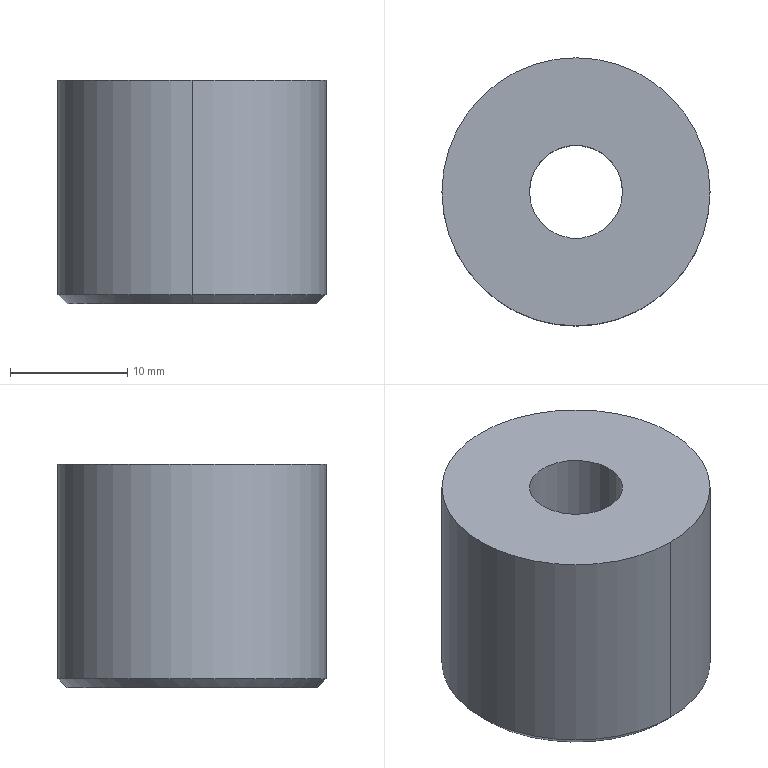Part | NX | features BREP 1 | 1 solid | 8 faces | box 22.86 x 22.86 x 19.05 mm | volume 6856 mm3 | cylinder 4 | plane 2 | cone 2 | commonest cylinder face diameters 7.938 x2 22.86 x2
STEP:
#1=CARTESIAN_POINT('',(0.,11.43,0.));
#2=VERTEX_POINT('',#1);
#3=CARTESIAN_POINT('',(0.,-11.43,0.));
#4=VERTEX_POINT('',#3);
#5=CARTESIAN_POINT('',(0.,0.,0.));
#6=DIRECTION('',(0.,0.,-1.));
#7=DIRECTION('',(0.,1.,0.));
#8=AXIS2_PLACEMENT_3D('',#5,#6,#7);
#9=CIRCLE('',#8,11.43);
#10=EDGE_CURVE('',#2,#4,#9,.T.);
#11=ORIENTED_EDGE('',*,*,#10,.F.);
#12=CARTESIAN_POINT('',(0.,0.,0.));
#13=DIRECTION('',(0.,0.,-1.));
#14=DIRECTION('',(0.,-1.,0.));
#15=AXIS2_PLACEMENT_3D('',#12,#13,#14);
#16=CIRCLE('',#15,11.43);
#17=EDGE_CURVE('',#4,#2,#16,.T.);
#18=ORIENTED_EDGE('',*,*,#17,.F.);
#19=EDGE_LOOP('',(#11,#18));
#20=FACE_BOUND('',#19,.T.);
#21=CARTESIAN_POINT('',(3.969,0.,0.));
#22=VERTEX_POINT('',#21);
#23=CARTESIAN_POINT('',(-3.969,0.,0.));
#24=VERTEX_POINT('',#23);
#25=CARTESIAN_POINT('',(0.,0.,0.));
#26=DIRECTION('',(0.,0.,-1.));
#27=DIRECTION('',(1.,0.,0.));
#28=AXIS2_PLACEMENT_3D('',#25,#26,#27);
#29=CIRCLE('',#28,3.969);
#30=EDGE_CURVE('',#22,#24,#29,.T.);
#31=ORIENTED_EDGE('',*,*,#30,.T.);
#32=CARTESIAN_POINT('',(0.,0.,0.));
#33=DIRECTION('',(0.,0.,-1.));
#34=DIRECTION('',(-1.,0.,0.));
#35=AXIS2_PLACEMENT_3D('',#32,#33,#34);
#36=CIRCLE('',#35,3.969);
#37=EDGE_CURVE('',#24,#22,#36,.T.);
#38=ORIENTED_EDGE('',*,*,#37,.T.);
#39=EDGE_LOOP('',(#31,#38));
#40=FACE_BOUND('',#39,.T.);
#41=CARTESIAN_POINT('',(0.,0.,0.));
#42=DIRECTION('',(0.,0.,-1.));
#43=DIRECTION('',(0.,-1.,0.));
#44=AXIS2_PLACEMENT_3D('',#41,#42,#43);
#45=PLANE('',#44);
#46=ADVANCED_FACE('',(#20,#40),#45,.F.);
#47=CARTESIAN_POINT('',(0.,11.43,-18.288));
#48=VERTEX_POINT('',#47);
#49=CARTESIAN_POINT('',(0.,11.43,0.));
#50=DIRECTION('',(0.,0.,-1.));
#51=VECTOR('',#50,1000.);
#52=LINE('',#49,#51);
#53=EDGE_CURVE('',#48,#2,#52,.F.);
#54=ORIENTED_EDGE('',*,*,#53,.F.);
#55=CARTESIAN_POINT('',(0.,-11.43,-18.288));
#56=VERTEX_POINT('',#55);
#57=CARTESIAN_POINT('',(0.,0.,-18.288));
#58=DIRECTION('',(0.,0.,-1.));
#59=DIRECTION('',(0.,-1.,0.));
#60=AXIS2_PLACEMENT_3D('',#57,#58,#59);
#61=CIRCLE('',#60,11.43);
#62=EDGE_CURVE('',#56,#48,#61,.T.);
#63=ORIENTED_EDGE('',*,*,#62,.F.);
#64=CARTESIAN_POINT('',(0.,-11.43,0.));
#65=DIRECTION('',(0.,0.,-1.));
#66=VECTOR('',#65,1000.);
#67=LINE('',#64,#66);
#68=EDGE_CURVE('',#56,#4,#67,.F.);
#69=ORIENTED_EDGE('',*,*,#68,.T.);
#70=ORIENTED_EDGE('',*,*,#17,.T.);
#71=EDGE_LOOP('',(#54,#63,#69,#70));
#72=FACE_BOUND('',#71,.T.);
#73=CARTESIAN_POINT('',(0.,0.,0.));
#74=DIRECTION('',(0.,0.,-1.));
#75=DIRECTION('',(0.,-1.,0.));
#76=AXIS2_PLACEMENT_3D('',#73,#74,#75);
#77=CYLINDRICAL_SURFACE('',#76,11.43);
#78=ADVANCED_FACE('',(#72),#77,.T.);
#79=ORIENTED_EDGE('',*,*,#68,.F.);
#80=CARTESIAN_POINT('',(0.,0.,-18.288));
#81=DIRECTION('',(0.,0.,-1.));
#82=DIRECTION('',(0.,1.,0.));
#83=AXIS2_PLACEMENT_3D('',#80,#81,#82);
#84=CIRCLE('',#83,11.43);
#85=EDGE_CURVE('',#48,#56,#84,.T.);
#86=ORIENTED_EDGE('',*,*,#85,.F.);
#87=ORIENTED_EDGE('',*,*,#53,.T.);
#88=ORIENTED_EDGE('',*,*,#10,.T.);
#89=EDGE_LOOP('',(#79,#86,#87,#88));
#90=FACE_BOUND('',#89,.T.);
#91=CARTESIAN_POINT('',(0.,0.,0.));
#92=DIRECTION('',(0.,0.,-1.));
#93=DIRECTION('',(0.,-1.,0.));
#94=AXIS2_PLACEMENT_3D('',#91,#92,#93);
#95=CYLINDRICAL_SURFACE('',#94,11.43);
#96=ADVANCED_FACE('',(#90),#95,.T.);
#97=CARTESIAN_POINT('',(0.,10.668,-19.05));
#98=VERTEX_POINT('',#97);
#99=CARTESIAN_POINT('',(0.,10.668,-19.05));
#100=DIRECTION('',(0.,0.7071,0.7071));
#101=VECTOR('',#100,1000.);
#102=LINE('',#99,#101);
#103=EDGE_CURVE('',#48,#98,#102,.F.);
#104=ORIENTED_EDGE('',*,*,#103,.F.);
#105=ORIENTED_EDGE('',*,*,#85,.T.);
#106=CARTESIAN_POINT('',(0.,-10.668,-19.05));
#107=VERTEX_POINT('',#106);
#108=CARTESIAN_POINT('',(0.,-10.668,-19.05));
#109=DIRECTION('',(0.,-0.7071,0.7071));
#110=VECTOR('',#109,1000.);
#111=LINE('',#108,#110);
#112=EDGE_CURVE('',#56,#107,#111,.F.);
#113=ORIENTED_EDGE('',*,*,#112,.T.);
#114=CARTESIAN_POINT('',(0.,0.,-19.05));
#115=DIRECTION('',(0.,0.,-1.));
#116=DIRECTION('',(0.,1.,0.));
#117=AXIS2_PLACEMENT_3D('',#114,#115,#116);
#118=CIRCLE('',#117,10.668);
#119=EDGE_CURVE('',#98,#107,#118,.T.);
#120=ORIENTED_EDGE('',*,*,#119,.F.);
#121=EDGE_LOOP('',(#104,#105,#113,#120));
#122=FACE_BOUND('',#121,.T.);
#123=CARTESIAN_POINT('',(0.,0.,-18.669));
#124=DIRECTION('',(0.,0.,1.));
#125=DIRECTION('',(0.,1.,0.));
#126=AXIS2_PLACEMENT_3D('',#123,#124,#125);
#127=CONICAL_SURFACE('',#126,11.049,0.7854);
#128=ADVANCED_FACE('',(#122),#127,.T.);
#129=ORIENTED_EDGE('',*,*,#119,.T.);
#130=CARTESIAN_POINT('',(0.,0.,-19.05));
#131=DIRECTION('',(0.,0.,-1.));
#132=DIRECTION('',(0.,-1.,0.));
#133=AXIS2_PLACEMENT_3D('',#130,#131,#132);
#134=CIRCLE('',#133,10.668);
#135=EDGE_CURVE('',#107,#98,#134,.T.);
#136=ORIENTED_EDGE('',*,*,#135,.T.);
#137=EDGE_LOOP('',(#129,#136));
#138=FACE_BOUND('',#137,.T.);
#139=CARTESIAN_POINT('',(3.969,0.,-19.05));
#140=VERTEX_POINT('',#139);
#141=CARTESIAN_POINT('',(-3.969,0.,-19.05));
#142=VERTEX_POINT('',#141);
#143=CARTESIAN_POINT('',(0.,0.,-19.05));
#144=DIRECTION('',(0.,0.,-1.));
#145=DIRECTION('',(1.,0.,0.));
#146=AXIS2_PLACEMENT_3D('',#143,#144,#145);
#147=CIRCLE('',#146,3.969);
#148=EDGE_CURVE('',#140,#142,#147,.T.);
#149=ORIENTED_EDGE('',*,*,#148,.F.);
#150=CARTESIAN_POINT('',(0.,0.,-19.05));
#151=DIRECTION('',(0.,0.,-1.));
#152=DIRECTION('',(-1.,0.,0.));
#153=AXIS2_PLACEMENT_3D('',#150,#151,#152);
#154=CIRCLE('',#153,3.969);
#155=EDGE_CURVE('',#142,#140,#154,.T.);
#156=ORIENTED_EDGE('',*,*,#155,.F.);
#157=EDGE_LOOP('',(#149,#156));
#158=FACE_BOUND('',#157,.T.);
#159=CARTESIAN_POINT('',(0.,0.,-19.05));
#160=DIRECTION('',(0.,0.,-1.));
#161=DIRECTION('',(0.,-1.,0.));
#162=AXIS2_PLACEMENT_3D('',#159,#160,#161);
#163=PLANE('',#162);
#164=ADVANCED_FACE('',(#138,#158),#163,.T.);
#165=ORIENTED_EDGE('',*,*,#112,.F.);
#166=ORIENTED_EDGE('',*,*,#62,.T.);
#167=ORIENTED_EDGE('',*,*,#103,.T.);
#168=ORIENTED_EDGE('',*,*,#135,.F.);
#169=EDGE_LOOP('',(#165,#166,#167,#168));
#170=FACE_BOUND('',#169,.T.);
#171=CARTESIAN_POINT('',(0.,0.,-18.669));
#172=DIRECTION('',(0.,0.,1.));
#173=DIRECTION('',(0.,1.,0.));
#174=AXIS2_PLACEMENT_3D('',#171,#172,#173);
#175=CONICAL_SURFACE('',#174,11.049,0.7854);
#176=ADVANCED_FACE('',(#170),#175,.T.);
#177=CARTESIAN_POINT('',(-3.969,0.,0.));
#178=DIRECTION('',(0.,0.,-1.));
#179=VECTOR('',#178,1000.);
#180=LINE('',#177,#179);
#181=EDGE_CURVE('',#24,#142,#180,.T.);
#182=ORIENTED_EDGE('',*,*,#181,.T.);
#183=ORIENTED_EDGE('',*,*,#155,.T.);
#184=CARTESIAN_POINT('',(3.969,0.,0.));
#185=DIRECTION('',(0.,0.,-1.));
#186=VECTOR('',#185,1000.);
#187=LINE('',#184,#186);
#188=EDGE_CURVE('',#22,#140,#187,.T.);
#189=ORIENTED_EDGE('',*,*,#188,.F.);
#190=ORIENTED_EDGE('',*,*,#37,.F.);
#191=EDGE_LOOP('',(#182,#183,#189,#190));
#192=FACE_BOUND('',#191,.T.);
#193=CARTESIAN_POINT('',(0.,0.,0.));
#194=DIRECTION('',(0.,0.,-1.));
#195=DIRECTION('',(-1.,0.,0.));
#196=AXIS2_PLACEMENT_3D('',#193,#194,#195);
#197=CYLINDRICAL_SURFACE('',#196,3.969);
#198=ADVANCED_FACE('',(#192),#197,.F.);
#199=ORIENTED_EDGE('',*,*,#188,.T.);
#200=ORIENTED_EDGE('',*,*,#148,.T.);
#201=ORIENTED_EDGE('',*,*,#181,.F.);
#202=ORIENTED_EDGE('',*,*,#30,.F.);
#203=EDGE_LOOP('',(#199,#200,#201,#202));
#204=FACE_BOUND('',#203,.T.);
#205=CARTESIAN_POINT('',(0.,0.,0.));
#206=DIRECTION('',(0.,0.,-1.));
#207=DIRECTION('',(-1.,0.,0.));
#208=AXIS2_PLACEMENT_3D('',#205,#206,#207);
#209=CYLINDRICAL_SURFACE('',#208,3.969);
#210=ADVANCED_FACE('',(#204),#209,.F.);
#211=CLOSED_SHELL('',(#46,#78,#96,#128,#164,#176,#198,#210));
#212=MANIFOLD_SOLID_BREP('',#211);
#213=(LENGTH_UNIT()NAMED_UNIT(*)SI_UNIT(.MILLI.,.METRE.));
#214=UNCERTAINTY_MEASURE_WITH_UNIT(LENGTH_MEASURE(0.00001),#213,'','');
#215=(NAMED_UNIT(*)PLANE_ANGLE_UNIT()SI_UNIT($,.RADIAN.));
#216=(NAMED_UNIT(*)SI_UNIT($,.STERADIAN.)SOLID_ANGLE_UNIT());
#217=(GEOMETRIC_REPRESENTATION_CONTEXT(3)GLOBAL_UNCERTAINTY_ASSIGNED_CONTEXT((#214))GLOBAL_UNIT_ASSIGNED_CONTEXT((#213,#215,#216))REPRESENTATION_CONTEXT('',''));
#218=ADVANCED_BREP_SHAPE_REPRESENTATION('',(#212),#217);